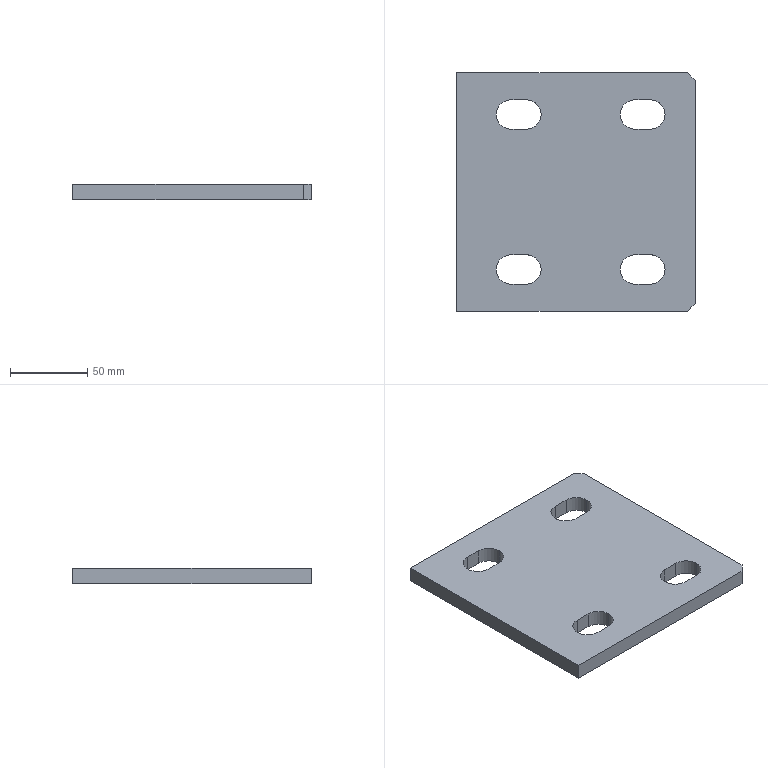Part | STEP file | 立柱翼Plate筋Plate-150 | 1 solid | 28 faces | box 154 x 154 x 10 mm | volume 217969 mm3 | plane 16 | cylinder 12 | commonest cylinder face diameters 19 x12